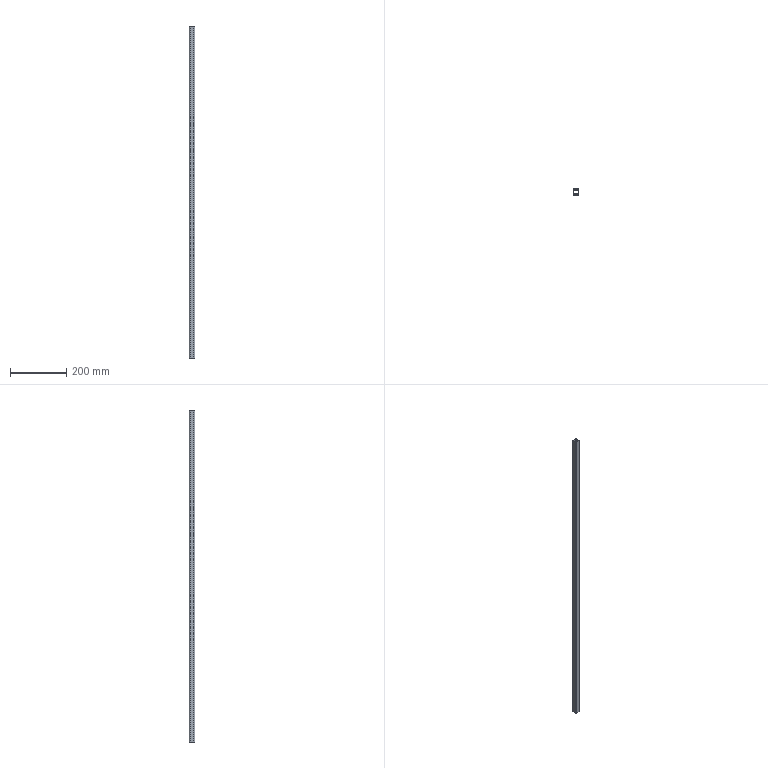Part | STEP file | DIN EN 10210-2 - 20 x 20 x 2 - 500 | 1 solid | 18 faces | box 20 x 20 x 1180 mm | volume 164855 mm3 | plane 10 | cylinder 8 | commonest cylinder face diameters 4 x4 6 x4
STEP:
#1=CARTESIAN_POINT('',(0.,0.,0.));
#2=DIRECTION('',(0.,0.,1.));
#3=DIRECTION('',(1.,0.,0.));
#4=AXIS2_PLACEMENT_3D('',#1,#2,#3);
#5=CARTESIAN_POINT('',(8.,6.,0.));
#6=VERTEX_POINT('',#5);
#7=CARTESIAN_POINT('',(8.,6.,1180.));
#8=VERTEX_POINT('',#7);
#9=CARTESIAN_POINT('',(8.,6.,0.));
#10=DIRECTION('',(0.,0.,1.));
#11=VECTOR('',#10,1.);
#12=LINE('',#9,#11);
#13=CARTESIAN_POINT('',(6.,6.,0.));
#14=DIRECTION('',(0.,0.,1.));
#15=DIRECTION('',(1.,0.,0.));
#16=AXIS2_PLACEMENT_3D('',#13,#14,#15);
#17=CYLINDRICAL_SURFACE('',#16,2.);
#18=CARTESIAN_POINT('',(0.,0.));
#19=DIRECTION('',(0.,1.));
#20=VECTOR('',#19,1.);
#21=LINE('',#18,#20);
#22=(GEOMETRIC_REPRESENTATION_CONTEXT(2)PARAMETRIC_REPRESENTATION_CONTEXT()REPRESENTATION_CONTEXT('',''));
#23=DEFINITIONAL_REPRESENTATION('',(#21),#22);
#24=PCURVE('',#17,#23);
#25=CARTESIAN_POINT('',(8.,6.,0.));
#26=DIRECTION('',(1.,0.,0.));
#27=DIRECTION('',(0.,0.,-1.));
#28=AXIS2_PLACEMENT_3D('',#25,#26,#27);
#29=PLANE('',#28);
#30=CARTESIAN_POINT('',(0.,0.));
#31=DIRECTION('',(-1.,0.));
#32=VECTOR('',#31,1.);
#33=LINE('',#30,#32);
#34=(GEOMETRIC_REPRESENTATION_CONTEXT(2)PARAMETRIC_REPRESENTATION_CONTEXT()REPRESENTATION_CONTEXT('',''));
#35=DEFINITIONAL_REPRESENTATION('',(#33),#34);
#36=PCURVE('',#29,#35);
#37=SURFACE_CURVE('',#12,(#24,#36),.PCURVE_S1.);
#38=EDGE_CURVE('',#6,#8,#37,.T.);
#39=ORIENTED_EDGE('',*,*,#38,.F.);
#40=CARTESIAN_POINT('',(6.,8.,0.));
#41=VERTEX_POINT('',#40);
#42=CARTESIAN_POINT('',(6.,6.,0.));
#43=DIRECTION('',(0.,0.,1.));
#44=DIRECTION('',(1.,0.,0.));
#45=AXIS2_PLACEMENT_3D('',#42,#43,#44);
#46=CIRCLE('',#45,2.);
#47=CARTESIAN_POINT('',(0.,0.));
#48=DIRECTION('',(1.,0.));
#49=VECTOR('',#48,1.);
#50=LINE('',#47,#49);
#51=(GEOMETRIC_REPRESENTATION_CONTEXT(2)PARAMETRIC_REPRESENTATION_CONTEXT()REPRESENTATION_CONTEXT('',''));
#52=DEFINITIONAL_REPRESENTATION('',(#50),#51);
#53=PCURVE('',#17,#52);
#54=CARTESIAN_POINT('',(0.,0.,0.));
#55=DIRECTION('',(0.,0.,1.));
#56=DIRECTION('',(1.,0.,0.));
#57=AXIS2_PLACEMENT_3D('',#54,#55,#56);
#58=PLANE('',#57);
#59=CARTESIAN_POINT('',(6.,6.));
#60=DIRECTION('',(1.,0.));
#61=AXIS2_PLACEMENT_2D('',#59,#60);
#62=CIRCLE('',#61,2.);
#63=(GEOMETRIC_REPRESENTATION_CONTEXT(2)PARAMETRIC_REPRESENTATION_CONTEXT()REPRESENTATION_CONTEXT('',''));
#64=DEFINITIONAL_REPRESENTATION('',(#62),#63);
#65=PCURVE('',#58,#64);
#66=SURFACE_CURVE('',#46,(#53,#65),.PCURVE_S1.);
#67=EDGE_CURVE('',#6,#41,#66,.T.);
#68=ORIENTED_EDGE('',*,*,#67,.T.);
#69=CARTESIAN_POINT('',(6.,8.,1180.));
#70=VERTEX_POINT('',#69);
#71=CARTESIAN_POINT('',(6.,8.,0.));
#72=DIRECTION('',(0.,0.,1.));
#73=VECTOR('',#72,1.);
#74=LINE('',#71,#73);
#75=CARTESIAN_POINT('',(1.571,0.));
#76=DIRECTION('',(0.,1.));
#77=VECTOR('',#76,1.);
#78=LINE('',#75,#77);
#79=(GEOMETRIC_REPRESENTATION_CONTEXT(2)PARAMETRIC_REPRESENTATION_CONTEXT()REPRESENTATION_CONTEXT('',''));
#80=DEFINITIONAL_REPRESENTATION('',(#78),#79);
#81=PCURVE('',#17,#80);
#82=CARTESIAN_POINT('',(-6.,8.,0.));
#83=DIRECTION('',(0.,1.,0.));
#84=DIRECTION('',(0.,0.,1.));
#85=AXIS2_PLACEMENT_3D('',#82,#83,#84);
#86=PLANE('',#85);
#87=CARTESIAN_POINT('',(0.,12.));
#88=DIRECTION('',(1.,0.));
#89=VECTOR('',#88,1.);
#90=LINE('',#87,#89);
#91=(GEOMETRIC_REPRESENTATION_CONTEXT(2)PARAMETRIC_REPRESENTATION_CONTEXT()REPRESENTATION_CONTEXT('',''));
#92=DEFINITIONAL_REPRESENTATION('',(#90),#91);
#93=PCURVE('',#86,#92);
#94=SURFACE_CURVE('',#74,(#81,#93),.PCURVE_S1.);
#95=EDGE_CURVE('',#41,#70,#94,.T.);
#96=ORIENTED_EDGE('',*,*,#95,.T.);
#97=CARTESIAN_POINT('',(6.,6.,1180.));
#98=DIRECTION('',(0.,0.,1.));
#99=DIRECTION('',(1.,0.,0.));
#100=AXIS2_PLACEMENT_3D('',#97,#98,#99);
#101=CIRCLE('',#100,2.);
#102=CARTESIAN_POINT('',(0.,1180.));
#103=DIRECTION('',(1.,0.));
#104=VECTOR('',#103,1.);
#105=LINE('',#102,#104);
#106=(GEOMETRIC_REPRESENTATION_CONTEXT(2)PARAMETRIC_REPRESENTATION_CONTEXT()REPRESENTATION_CONTEXT('',''));
#107=DEFINITIONAL_REPRESENTATION('',(#105),#106);
#108=PCURVE('',#17,#107);
#109=CARTESIAN_POINT('',(0.,0.,1180.));
#110=DIRECTION('',(0.,0.,1.));
#111=DIRECTION('',(1.,0.,0.));
#112=AXIS2_PLACEMENT_3D('',#109,#110,#111);
#113=PLANE('',#112);
#114=CARTESIAN_POINT('',(6.,6.));
#115=DIRECTION('',(1.,0.));
#116=AXIS2_PLACEMENT_2D('',#114,#115);
#117=CIRCLE('',#116,2.);
#118=(GEOMETRIC_REPRESENTATION_CONTEXT(2)PARAMETRIC_REPRESENTATION_CONTEXT()REPRESENTATION_CONTEXT('',''));
#119=DEFINITIONAL_REPRESENTATION('',(#117),#118);
#120=PCURVE('',#113,#119);
#121=SURFACE_CURVE('',#101,(#108,#120),.PCURVE_S1.);
#122=EDGE_CURVE('',#8,#70,#121,.T.);
#123=ORIENTED_EDGE('',*,*,#122,.F.);
#124=EDGE_LOOP('',(#39,#68,#96,#123));
#125=FACE_BOUND('',#124,.F.);
#126=ADVANCED_FACE('',(#125),#17,.F.);
#127=CARTESIAN_POINT('',(-6.,8.,1180.));
#128=VERTEX_POINT('',#127);
#129=CARTESIAN_POINT('',(-3.,8.,1180.));
#130=DIRECTION('',(-1.,0.,0.));
#131=VECTOR('',#130,1.);
#132=LINE('',#129,#131);
#133=CARTESIAN_POINT('',(1180.,3.));
#134=DIRECTION('',(0.,-1.));
#135=VECTOR('',#134,1.);
#136=LINE('',#133,#135);
#137=(GEOMETRIC_REPRESENTATION_CONTEXT(2)PARAMETRIC_REPRESENTATION_CONTEXT()REPRESENTATION_CONTEXT('',''));
#138=DEFINITIONAL_REPRESENTATION('',(#136),#137);
#139=PCURVE('',#86,#138);
#140=CARTESIAN_POINT('',(-3.,8.));
#141=DIRECTION('',(-1.,0.));
#142=VECTOR('',#141,1.);
#143=LINE('',#140,#142);
#144=(GEOMETRIC_REPRESENTATION_CONTEXT(2)PARAMETRIC_REPRESENTATION_CONTEXT()REPRESENTATION_CONTEXT('',''));
#145=DEFINITIONAL_REPRESENTATION('',(#143),#144);
#146=PCURVE('',#113,#145);
#147=SURFACE_CURVE('',#132,(#139,#146),.PCURVE_S1.);
#148=EDGE_CURVE('',#70,#128,#147,.T.);
#149=ORIENTED_EDGE('',*,*,#148,.T.);
#150=CARTESIAN_POINT('',(-6.,8.,0.));
#151=VERTEX_POINT('',#150);
#152=CARTESIAN_POINT('',(-6.,8.,0.));
#153=DIRECTION('',(0.,0.,1.));
#154=VECTOR('',#153,1.);
#155=LINE('',#152,#154);
#156=CARTESIAN_POINT('',(0.,0.));
#157=DIRECTION('',(1.,0.));
#158=VECTOR('',#157,1.);
#159=LINE('',#156,#158);
#160=(GEOMETRIC_REPRESENTATION_CONTEXT(2)PARAMETRIC_REPRESENTATION_CONTEXT()REPRESENTATION_CONTEXT('',''));
#161=DEFINITIONAL_REPRESENTATION('',(#159),#160);
#162=PCURVE('',#86,#161);
#163=CARTESIAN_POINT('',(-6.,6.,0.));
#164=DIRECTION('',(0.,0.,1.));
#165=DIRECTION('',(0.,1.,0.));
#166=AXIS2_PLACEMENT_3D('',#163,#164,#165);
#167=CYLINDRICAL_SURFACE('',#166,2.);
#168=CARTESIAN_POINT('',(0.,0.));
#169=DIRECTION('',(0.,1.));
#170=VECTOR('',#169,1.);
#171=LINE('',#168,#170);
#172=(GEOMETRIC_REPRESENTATION_CONTEXT(2)PARAMETRIC_REPRESENTATION_CONTEXT()REPRESENTATION_CONTEXT('',''));
#173=DEFINITIONAL_REPRESENTATION('',(#171),#172);
#174=PCURVE('',#167,#173);
#175=SURFACE_CURVE('',#155,(#162,#174),.PCURVE_S1.);
#176=EDGE_CURVE('',#151,#128,#175,.T.);
#177=ORIENTED_EDGE('',*,*,#176,.F.);
#178=CARTESIAN_POINT('',(-3.,8.,0.));
#179=DIRECTION('',(-1.,0.,0.));
#180=VECTOR('',#179,1.);
#181=LINE('',#178,#180);
#182=CARTESIAN_POINT('',(0.,3.));
#183=DIRECTION('',(0.,-1.));
#184=VECTOR('',#183,1.);
#185=LINE('',#182,#184);
#186=(GEOMETRIC_REPRESENTATION_CONTEXT(2)PARAMETRIC_REPRESENTATION_CONTEXT()REPRESENTATION_CONTEXT('',''));
#187=DEFINITIONAL_REPRESENTATION('',(#185),#186);
#188=PCURVE('',#86,#187);
#189=CARTESIAN_POINT('',(-3.,8.));
#190=DIRECTION('',(-1.,0.));
#191=VECTOR('',#190,1.);
#192=LINE('',#189,#191);
#193=(GEOMETRIC_REPRESENTATION_CONTEXT(2)PARAMETRIC_REPRESENTATION_CONTEXT()REPRESENTATION_CONTEXT('',''));
#194=DEFINITIONAL_REPRESENTATION('',(#192),#193);
#195=PCURVE('',#58,#194);
#196=SURFACE_CURVE('',#181,(#188,#195),.PCURVE_S1.);
#197=EDGE_CURVE('',#41,#151,#196,.T.);
#198=ORIENTED_EDGE('',*,*,#197,.F.);
#199=ORIENTED_EDGE('',*,*,#95,.T.);
#200=EDGE_LOOP('',(#149,#177,#198,#199));
#201=FACE_BOUND('',#200,.T.);
#202=ADVANCED_FACE('',(#201),#86,.F.);
#203=ORIENTED_EDGE('',*,*,#176,.F.);
#204=CARTESIAN_POINT('',(-8.,6.,0.));
#205=VERTEX_POINT('',#204);
#206=CARTESIAN_POINT('',(-6.,6.,0.));
#207=DIRECTION('',(0.,0.,1.));
#208=DIRECTION('',(0.,1.,0.));
#209=AXIS2_PLACEMENT_3D('',#206,#207,#208);
#210=CIRCLE('',#209,2.);
#211=CARTESIAN_POINT('',(0.,0.));
#212=DIRECTION('',(1.,0.));
#213=VECTOR('',#212,1.);
#214=LINE('',#211,#213);
#215=(GEOMETRIC_REPRESENTATION_CONTEXT(2)PARAMETRIC_REPRESENTATION_CONTEXT()REPRESENTATION_CONTEXT('',''));
#216=DEFINITIONAL_REPRESENTATION('',(#214),#215);
#217=PCURVE('',#167,#216);
#218=CARTESIAN_POINT('',(-6.,6.));
#219=DIRECTION('',(0.,1.));
#220=AXIS2_PLACEMENT_2D('',#218,#219);
#221=CIRCLE('',#220,2.);
#222=(GEOMETRIC_REPRESENTATION_CONTEXT(2)PARAMETRIC_REPRESENTATION_CONTEXT()REPRESENTATION_CONTEXT('',''));
#223=DEFINITIONAL_REPRESENTATION('',(#221),#222);
#224=PCURVE('',#58,#223);
#225=SURFACE_CURVE('',#210,(#217,#224),.PCURVE_S1.);
#226=EDGE_CURVE('',#151,#205,#225,.T.);
#227=ORIENTED_EDGE('',*,*,#226,.T.);
#228=CARTESIAN_POINT('',(-8.,6.,1180.));
#229=VERTEX_POINT('',#228);
#230=CARTESIAN_POINT('',(-8.,6.,0.));
#231=DIRECTION('',(0.,0.,1.));
#232=VECTOR('',#231,1.);
#233=LINE('',#230,#232);
#234=CARTESIAN_POINT('',(1.571,0.));
#235=DIRECTION('',(0.,1.));
#236=VECTOR('',#235,1.);
#237=LINE('',#234,#236);
#238=(GEOMETRIC_REPRESENTATION_CONTEXT(2)PARAMETRIC_REPRESENTATION_CONTEXT()REPRESENTATION_CONTEXT('',''));
#239=DEFINITIONAL_REPRESENTATION('',(#237),#238);
#240=PCURVE('',#167,#239);
#241=CARTESIAN_POINT('',(-8.,-6.,0.));
#242=DIRECTION('',(-1.,0.,0.));
#243=DIRECTION('',(0.,0.,1.));
#244=AXIS2_PLACEMENT_3D('',#241,#242,#243);
#245=PLANE('',#244);
#246=CARTESIAN_POINT('',(0.,12.));
#247=DIRECTION('',(1.,0.));
#248=VECTOR('',#247,1.);
#249=LINE('',#246,#248);
#250=(GEOMETRIC_REPRESENTATION_CONTEXT(2)PARAMETRIC_REPRESENTATION_CONTEXT()REPRESENTATION_CONTEXT('',''));
#251=DEFINITIONAL_REPRESENTATION('',(#249),#250);
#252=PCURVE('',#245,#251);
#253=SURFACE_CURVE('',#233,(#240,#252),.PCURVE_S1.);
#254=EDGE_CURVE('',#205,#229,#253,.T.);
#255=ORIENTED_EDGE('',*,*,#254,.T.);
#256=CARTESIAN_POINT('',(-6.,6.,1180.));
#257=DIRECTION('',(0.,0.,1.));
#258=DIRECTION('',(0.,1.,0.));
#259=AXIS2_PLACEMENT_3D('',#256,#257,#258);
#260=CIRCLE('',#259,2.);
#261=CARTESIAN_POINT('',(0.,1180.));
#262=DIRECTION('',(1.,0.));
#263=VECTOR('',#262,1.);
#264=LINE('',#261,#263);
#265=(GEOMETRIC_REPRESENTATION_CONTEXT(2)PARAMETRIC_REPRESENTATION_CONTEXT()REPRESENTATION_CONTEXT('',''));
#266=DEFINITIONAL_REPRESENTATION('',(#264),#265);
#267=PCURVE('',#167,#266);
#268=CARTESIAN_POINT('',(-6.,6.));
#269=DIRECTION('',(0.,1.));
#270=AXIS2_PLACEMENT_2D('',#268,#269);
#271=CIRCLE('',#270,2.);
#272=(GEOMETRIC_REPRESENTATION_CONTEXT(2)PARAMETRIC_REPRESENTATION_CONTEXT()REPRESENTATION_CONTEXT('',''));
#273=DEFINITIONAL_REPRESENTATION('',(#271),#272);
#274=PCURVE('',#113,#273);
#275=SURFACE_CURVE('',#260,(#267,#274),.PCURVE_S1.);
#276=EDGE_CURVE('',#128,#229,#275,.T.);
#277=ORIENTED_EDGE('',*,*,#276,.F.);
#278=EDGE_LOOP('',(#203,#227,#255,#277));
#279=FACE_BOUND('',#278,.F.);
#280=ADVANCED_FACE('',(#279),#167,.F.);
#281=CARTESIAN_POINT('',(-8.,-6.,1180.));
#282=VERTEX_POINT('',#281);
#283=CARTESIAN_POINT('',(-8.,-3.,1180.));
#284=DIRECTION('',(0.,-1.,0.));
#285=VECTOR('',#284,1.);
#286=LINE('',#283,#285);
#287=CARTESIAN_POINT('',(1180.,3.));
#288=DIRECTION('',(0.,-1.));
#289=VECTOR('',#288,1.);
#290=LINE('',#287,#289);
#291=(GEOMETRIC_REPRESENTATION_CONTEXT(2)PARAMETRIC_REPRESENTATION_CONTEXT()REPRESENTATION_CONTEXT('',''));
#292=DEFINITIONAL_REPRESENTATION('',(#290),#291);
#293=PCURVE('',#245,#292);
#294=CARTESIAN_POINT('',(-8.,-3.));
#295=DIRECTION('',(0.,-1.));
#296=VECTOR('',#295,1.);
#297=LINE('',#294,#296);
#298=(GEOMETRIC_REPRESENTATION_CONTEXT(2)PARAMETRIC_REPRESENTATION_CONTEXT()REPRESENTATION_CONTEXT('',''));
#299=DEFINITIONAL_REPRESENTATION('',(#297),#298);
#300=PCURVE('',#113,#299);
#301=SURFACE_CURVE('',#286,(#293,#300),.PCURVE_S1.);
#302=EDGE_CURVE('',#229,#282,#301,.T.);
#303=ORIENTED_EDGE('',*,*,#302,.T.);
#304=CARTESIAN_POINT('',(-8.,-6.,0.));
#305=VERTEX_POINT('',#304);
#306=CARTESIAN_POINT('',(-8.,-6.,0.));
#307=DIRECTION('',(0.,0.,1.));
#308=VECTOR('',#307,1.);
#309=LINE('',#306,#308);
#310=CARTESIAN_POINT('',(0.,0.));
#311=DIRECTION('',(1.,0.));
#312=VECTOR('',#311,1.);
#313=LINE('',#310,#312);
#314=(GEOMETRIC_REPRESENTATION_CONTEXT(2)PARAMETRIC_REPRESENTATION_CONTEXT()REPRESENTATION_CONTEXT('',''));
#315=DEFINITIONAL_REPRESENTATION('',(#313),#314);
#316=PCURVE('',#245,#315);
#317=CARTESIAN_POINT('',(-6.,-6.,0.));
#318=DIRECTION('',(0.,0.,1.));
#319=DIRECTION('',(-1.,0.,0.));
#320=AXIS2_PLACEMENT_3D('',#317,#318,#319);
#321=CYLINDRICAL_SURFACE('',#320,2.);
#322=CARTESIAN_POINT('',(0.,0.));
#323=DIRECTION('',(0.,1.));
#324=VECTOR('',#323,1.);
#325=LINE('',#322,#324);
#326=(GEOMETRIC_REPRESENTATION_CONTEXT(2)PARAMETRIC_REPRESENTATION_CONTEXT()REPRESENTATION_CONTEXT('',''));
#327=DEFINITIONAL_REPRESENTATION('',(#325),#326);
#328=PCURVE('',#321,#327);
#329=SURFACE_CURVE('',#309,(#316,#328),.PCURVE_S1.);
#330=EDGE_CURVE('',#305,#282,#329,.T.);
#331=ORIENTED_EDGE('',*,*,#330,.F.);
#332=CARTESIAN_POINT('',(-8.,-3.,0.));
#333=DIRECTION('',(0.,-1.,0.));
#334=VECTOR('',#333,1.);
#335=LINE('',#332,#334);
#336=CARTESIAN_POINT('',(0.,3.));
#337=DIRECTION('',(0.,-1.));
#338=VECTOR('',#337,1.);
#339=LINE('',#336,#338);
#340=(GEOMETRIC_REPRESENTATION_CONTEXT(2)PARAMETRIC_REPRESENTATION_CONTEXT()REPRESENTATION_CONTEXT('',''));
#341=DEFINITIONAL_REPRESENTATION('',(#339),#340);
#342=PCURVE('',#245,#341);
#343=CARTESIAN_POINT('',(-8.,-3.));
#344=DIRECTION('',(0.,-1.));
#345=VECTOR('',#344,1.);
#346=LINE('',#343,#345);
#347=(GEOMETRIC_REPRESENTATION_CONTEXT(2)PARAMETRIC_REPRESENTATION_CONTEXT()REPRESENTATION_CONTEXT('',''));
#348=DEFINITIONAL_REPRESENTATION('',(#346),#347);
#349=PCURVE('',#58,#348);
#350=SURFACE_CURVE('',#335,(#342,#349),.PCURVE_S1.);
#351=EDGE_CURVE('',#205,#305,#350,.T.);
#352=ORIENTED_EDGE('',*,*,#351,.F.);
#353=ORIENTED_EDGE('',*,*,#254,.T.);
#354=EDGE_LOOP('',(#303,#331,#352,#353));
#355=FACE_BOUND('',#354,.T.);
#356=ADVANCED_FACE('',(#355),#245,.F.);
#357=CARTESIAN_POINT('',(10.,7.,1180.));
#358=VERTEX_POINT('',#357);
#359=CARTESIAN_POINT('',(10.,-7.,1180.));
#360=VERTEX_POINT('',#359);
#361=CARTESIAN_POINT('',(10.,3.5,1180.));
#362=DIRECTION('',(0.,-1.,0.));
#363=VECTOR('',#362,1.);
#364=LINE('',#361,#363);
#365=CARTESIAN_POINT('',(10.,7.,0.));
#366=DIRECTION('',(1.,0.,0.));
#367=DIRECTION('',(0.,0.,-1.));
#368=AXIS2_PLACEMENT_3D('',#365,#366,#367);
#369=PLANE('',#368);
#370=CARTESIAN_POINT('',(-1180.,-3.5));
#371=DIRECTION('',(0.,-1.));
#372=VECTOR('',#371,1.);
#373=LINE('',#370,#372);
#374=(GEOMETRIC_REPRESENTATION_CONTEXT(2)PARAMETRIC_REPRESENTATION_CONTEXT()REPRESENTATION_CONTEXT('',''));
#375=DEFINITIONAL_REPRESENTATION('',(#373),#374);
#376=PCURVE('',#369,#375);
#377=CARTESIAN_POINT('',(10.,3.5));
#378=DIRECTION('',(0.,-1.));
#379=VECTOR('',#378,1.);
#380=LINE('',#377,#379);
#381=(GEOMETRIC_REPRESENTATION_CONTEXT(2)PARAMETRIC_REPRESENTATION_CONTEXT()REPRESENTATION_CONTEXT('',''));
#382=DEFINITIONAL_REPRESENTATION('',(#380),#381);
#383=PCURVE('',#113,#382);
#384=SURFACE_CURVE('',#364,(#376,#383),.PCURVE_S1.);
#385=EDGE_CURVE('',#358,#360,#384,.T.);
#386=ORIENTED_EDGE('',*,*,#385,.T.);
#387=CARTESIAN_POINT('',(10.,-7.,0.));
#388=VERTEX_POINT('',#387);
#389=CARTESIAN_POINT('',(10.,-7.,0.));
#390=DIRECTION('',(0.,0.,1.));
#391=VECTOR('',#390,1.);
#392=LINE('',#389,#391);
#393=CARTESIAN_POINT('',(0.,-14.));
#394=DIRECTION('',(-1.,0.));
#395=VECTOR('',#394,1.);
#396=LINE('',#393,#395);
#397=(GEOMETRIC_REPRESENTATION_CONTEXT(2)PARAMETRIC_REPRESENTATION_CONTEXT()REPRESENTATION_CONTEXT('',''));
#398=DEFINITIONAL_REPRESENTATION('',(#396),#397);
#399=PCURVE('',#369,#398);
#400=CARTESIAN_POINT('',(7.,-7.,0.));
#401=DIRECTION('',(0.,0.,1.));
#402=DIRECTION('',(0.,1.,0.));
#403=AXIS2_PLACEMENT_3D('',#400,#401,#402);
#404=CYLINDRICAL_SURFACE('',#403,3.);
#405=CARTESIAN_POINT('',(4.712,0.));
#406=DIRECTION('',(0.,1.));
#407=VECTOR('',#406,1.);
#408=LINE('',#405,#407);
#409=(GEOMETRIC_REPRESENTATION_CONTEXT(2)PARAMETRIC_REPRESENTATION_CONTEXT()REPRESENTATION_CONTEXT('',''));
#410=DEFINITIONAL_REPRESENTATION('',(#408),#409);
#411=PCURVE('',#404,#410);
#412=SURFACE_CURVE('',#392,(#399,#411),.PCURVE_S1.);
#413=EDGE_CURVE('',#388,#360,#412,.T.);
#414=ORIENTED_EDGE('',*,*,#413,.F.);
#415=CARTESIAN_POINT('',(10.,7.,0.));
#416=VERTEX_POINT('',#415);
#417=CARTESIAN_POINT('',(10.,3.5,0.));
#418=DIRECTION('',(0.,-1.,0.));
#419=VECTOR('',#418,1.);
#420=LINE('',#417,#419);
#421=CARTESIAN_POINT('',(0.,-3.5));
#422=DIRECTION('',(0.,-1.));
#423=VECTOR('',#422,1.);
#424=LINE('',#421,#423);
#425=(GEOMETRIC_REPRESENTATION_CONTEXT(2)PARAMETRIC_REPRESENTATION_CONTEXT()REPRESENTATION_CONTEXT('',''));
#426=DEFINITIONAL_REPRESENTATION('',(#424),#425);
#427=PCURVE('',#369,#426);
#428=CARTESIAN_POINT('',(10.,3.5));
#429=DIRECTION('',(0.,-1.));
#430=VECTOR('',#429,1.);
#431=LINE('',#428,#430);
#432=(GEOMETRIC_REPRESENTATION_CONTEXT(2)PARAMETRIC_REPRESENTATION_CONTEXT()REPRESENTATION_CONTEXT('',''));
#433=DEFINITIONAL_REPRESENTATION('',(#431),#432);
#434=PCURVE('',#58,#433);
#435=SURFACE_CURVE('',#420,(#427,#434),.PCURVE_S1.);
#436=EDGE_CURVE('',#416,#388,#435,.T.);
#437=ORIENTED_EDGE('',*,*,#436,.F.);
#438=CARTESIAN_POINT('',(10.,7.,0.));
#439=DIRECTION('',(0.,0.,1.));
#440=VECTOR('',#439,1.);
#441=LINE('',#438,#440);
#442=CARTESIAN_POINT('',(0.,0.));
#443=DIRECTION('',(-1.,0.));
#444=VECTOR('',#443,1.);
#445=LINE('',#442,#444);
#446=(GEOMETRIC_REPRESENTATION_CONTEXT(2)PARAMETRIC_REPRESENTATION_CONTEXT()REPRESENTATION_CONTEXT('',''));
#447=DEFINITIONAL_REPRESENTATION('',(#445),#446);
#448=PCURVE('',#369,#447);
#449=CARTESIAN_POINT('',(7.,7.,0.));
#450=DIRECTION('',(0.,0.,1.));
#451=DIRECTION('',(-1.,0.,0.));
#452=AXIS2_PLACEMENT_3D('',#449,#450,#451);
#453=CYLINDRICAL_SURFACE('',#452,3.);
#454=CARTESIAN_POINT('',(3.142,0.));
#455=DIRECTION('',(0.,1.));
#456=VECTOR('',#455,1.);
#457=LINE('',#454,#456);
#458=(GEOMETRIC_REPRESENTATION_CONTEXT(2)PARAMETRIC_REPRESENTATION_CONTEXT()REPRESENTATION_CONTEXT('',''));
#459=DEFINITIONAL_REPRESENTATION('',(#457),#458);
#460=PCURVE('',#453,#459);
#461=SURFACE_CURVE('',#441,(#448,#460),.PCURVE_S1.);
#462=EDGE_CURVE('',#416,#358,#461,.T.);
#463=ORIENTED_EDGE('',*,*,#462,.T.);
#464=EDGE_LOOP('',(#386,#414,#437,#463));
#465=FACE_BOUND('',#464,.T.);
#466=ADVANCED_FACE('',(#465),#369,.T.);
#467=CARTESIAN_POINT('',(7.,-10.,1180.));
#468=VERTEX_POINT('',#467);
#469=CARTESIAN_POINT('',(7.,-7.,1180.));
#470=DIRECTION('',(0.,0.,-1.));
#471=DIRECTION('',(0.,1.,0.));
#472=AXIS2_PLACEMENT_3D('',#469,#470,#471);
#473=CIRCLE('',#472,3.);
#474=CARTESIAN_POINT('',(6.283,1180.));
#475=DIRECTION('',(-1.,0.));
#476=VECTOR('',#475,1.);
#477=LINE('',#474,#476);
#478=(GEOMETRIC_REPRESENTATION_CONTEXT(2)PARAMETRIC_REPRESENTATION_CONTEXT()REPRESENTATION_CONTEXT('',''));
#479=DEFINITIONAL_REPRESENTATION('',(#477),#478);
#480=PCURVE('',#404,#479);
#481=CARTESIAN_POINT('',(7.,-4.));
#482=CARTESIAN_POINT('',(12.196,-4.));
#483=CARTESIAN_POINT('',(9.598,-8.5));
#484=CARTESIAN_POINT('',(7.,-13.));
#485=CARTESIAN_POINT('',(4.402,-8.5));
#486=CARTESIAN_POINT('',(1.804,-4.));
#487=CARTESIAN_POINT('',(7.,-4.));
#488=(BOUNDED_CURVE()B_SPLINE_CURVE(2,(#481,#482,#483,#484,#485,#486,#487),.UNSPECIFIED.,.T.,.F.)B_SPLINE_CURVE_WITH_KNOTS((1,2,2,2,2,1),(-2.094,0.,2.094,4.189,6.283,8.378),.UNSPECIFIED.)CURVE()GEOMETRIC_REPRESENTATION_ITEM()RATIONAL_B_SPLINE_CURVE((1.,0.5,1.,0.5,1.,0.5,1.))REPRESENTATION_ITEM(''));
#489=(GEOMETRIC_REPRESENTATION_CONTEXT(2)PARAMETRIC_REPRESENTATION_CONTEXT()REPRESENTATION_CONTEXT('',''));
#490=DEFINITIONAL_REPRESENTATION('',(#488),#489);
#491=PCURVE('',#113,#490);
#492=SURFACE_CURVE('',#473,(#480,#491),.PCURVE_S1.);
#493=EDGE_CURVE('',#360,#468,#492,.T.);
#494=ORIENTED_EDGE('',*,*,#493,.T.);
#495=CARTESIAN_POINT('',(7.,-10.,0.));
#496=VERTEX_POINT('',#495);
#497=CARTESIAN_POINT('',(7.,-10.,0.));
#498=DIRECTION('',(0.,0.,1.));
#499=VECTOR('',#498,1.);
#500=LINE('',#497,#499);
#501=CARTESIAN_POINT('',(3.142,0.));
#502=DIRECTION('',(0.,1.));
#503=VECTOR('',#502,1.);
#504=LINE('',#501,#503);
#505=(GEOMETRIC_REPRESENTATION_CONTEXT(2)PARAMETRIC_REPRESENTATION_CONTEXT()REPRESENTATION_CONTEXT('',''));
#506=DEFINITIONAL_REPRESENTATION('',(#504),#505);
#507=PCURVE('',#404,#506);
#508=CARTESIAN_POINT('',(7.,-10.,0.));
#509=DIRECTION('',(0.,-1.,0.));
#510=DIRECTION('',(0.,0.,-1.));
#511=AXIS2_PLACEMENT_3D('',#508,#509,#510);
#512=PLANE('',#511);
#513=CARTESIAN_POINT('',(0.,0.));
#514=DIRECTION('',(-1.,0.));
#515=VECTOR('',#514,1.);
#516=LINE('',#513,#515);
#517=(GEOMETRIC_REPRESENTATION_CONTEXT(2)PARAMETRIC_REPRESENTATION_CONTEXT()REPRESENTATION_CONTEXT('',''));
#518=DEFINITIONAL_REPRESENTATION('',(#516),#517);
#519=PCURVE('',#512,#518);
#520=SURFACE_CURVE('',#500,(#507,#519),.PCURVE_S1.);
#521=EDGE_CURVE('',#496,#468,#520,.T.);
#522=ORIENTED_EDGE('',*,*,#521,.F.);
#523=CARTESIAN_POINT('',(7.,-7.,0.));
#524=DIRECTION('',(0.,0.,-1.));
#525=DIRECTION('',(0.,1.,0.));
#526=AXIS2_PLACEMENT_3D('',#523,#524,#525);
#527=CIRCLE('',#526,3.);
#528=CARTESIAN_POINT('',(6.283,0.));
#529=DIRECTION('',(-1.,0.));
#530=VECTOR('',#529,1.);
#531=LINE('',#528,#530);
#532=(GEOMETRIC_REPRESENTATION_CONTEXT(2)PARAMETRIC_REPRESENTATION_CONTEXT()REPRESENTATION_CONTEXT('',''));
#533=DEFINITIONAL_REPRESENTATION('',(#531),#532);
#534=PCURVE('',#404,#533);
#535=CARTESIAN_POINT('',(7.,-4.));
#536=CARTESIAN_POINT('',(12.196,-4.));
#537=CARTESIAN_POINT('',(9.598,-8.5));
#538=CARTESIAN_POINT('',(7.,-13.));
#539=CARTESIAN_POINT('',(4.402,-8.5));
#540=CARTESIAN_POINT('',(1.804,-4.));
#541=CARTESIAN_POINT('',(7.,-4.));
#542=(BOUNDED_CURVE()B_SPLINE_CURVE(2,(#535,#536,#537,#538,#539,#540,#541),.UNSPECIFIED.,.T.,.F.)B_SPLINE_CURVE_WITH_KNOTS((1,2,2,2,2,1),(-2.094,0.,2.094,4.189,6.283,8.378),.UNSPECIFIED.)CURVE()GEOMETRIC_REPRESENTATION_ITEM()RATIONAL_B_SPLINE_CURVE((1.,0.5,1.,0.5,1.,0.5,1.))REPRESENTATION_ITEM(''));
#543=(GEOMETRIC_REPRESENTATION_CONTEXT(2)PARAMETRIC_REPRESENTATION_CONTEXT()REPRESENTATION_CONTEXT('',''));
#544=DEFINITIONAL_REPRESENTATION('',(#542),#543);
#545=PCURVE('',#58,#544);
#546=SURFACE_CURVE('',#527,(#534,#545),.PCURVE_S1.);
#547=EDGE_CURVE('',#388,#496,#546,.T.);
#548=ORIENTED_EDGE('',*,*,#547,.F.);
#549=ORIENTED_EDGE('',*,*,#413,.T.);
#550=EDGE_LOOP('',(#494,#522,#548,#549));
#551=FACE_BOUND('',#550,.T.);
#552=ADVANCED_FACE('',(#551),#404,.T.);
#553=CARTESIAN_POINT('',(-7.,-10.,1180.));
#554=VERTEX_POINT('',#553);
#555=CARTESIAN_POINT('',(3.5,-10.,1180.));
#556=DIRECTION('',(-1.,0.,0.));
#557=VECTOR('',#556,1.);
#558=LINE('',#555,#557);
#559=CARTESIAN_POINT('',(-1180.,-3.5));
#560=DIRECTION('',(0.,-1.));
#561=VECTOR('',#560,1.);
#562=LINE('',#559,#561);
#563=(GEOMETRIC_REPRESENTATION_CONTEXT(2)PARAMETRIC_REPRESENTATION_CONTEXT()REPRESENTATION_CONTEXT('',''));
#564=DEFINITIONAL_REPRESENTATION('',(#562),#563);
#565=PCURVE('',#512,#564);
#566=CARTESIAN_POINT('',(3.5,-10.));
#567=DIRECTION('',(-1.,0.));
#568=VECTOR('',#567,1.);
#569=LINE('',#566,#568);
#570=(GEOMETRIC_REPRESENTATION_CONTEXT(2)PARAMETRIC_REPRESENTATION_CONTEXT()REPRESENTATION_CONTEXT('',''));
#571=DEFINITIONAL_REPRESENTATION('',(#569),#570);
#572=PCURVE('',#113,#571);
#573=SURFACE_CURVE('',#558,(#565,#572),.PCURVE_S1.);
#574=EDGE_CURVE('',#468,#554,#573,.T.);
#575=ORIENTED_EDGE('',*,*,#574,.T.);
#576=CARTESIAN_POINT('',(-7.,-10.,0.));
#577=VERTEX_POINT('',#576);
#578=CARTESIAN_POINT('',(-7.,-10.,0.));
#579=DIRECTION('',(0.,0.,1.));
#580=VECTOR('',#579,1.);
#581=LINE('',#578,#580);
#582=CARTESIAN_POINT('',(0.,-14.));
#583=DIRECTION('',(-1.,0.));
#584=VECTOR('',#583,1.);
#585=LINE('',#582,#584);
#586=(GEOMETRIC_REPRESENTATION_CONTEXT(2)PARAMETRIC_REPRESENTATION_CONTEXT()REPRESENTATION_CONTEXT('',''));
#587=DEFINITIONAL_REPRESENTATION('',(#585),#586);
#588=PCURVE('',#512,#587);
#589=CARTESIAN_POINT('',(-7.,-7.,0.));
#590=DIRECTION('',(0.,0.,1.));
#591=DIRECTION('',(1.,0.,0.));
#592=AXIS2_PLACEMENT_3D('',#589,#590,#591);
#593=CYLINDRICAL_SURFACE('',#592,3.);
#594=CARTESIAN_POINT('',(4.712,0.));
#595=DIRECTION('',(0.,1.));
#596=VECTOR('',#595,1.);
#597=LINE('',#594,#596);
#598=(GEOMETRIC_REPRESENTATION_CONTEXT(2)PARAMETRIC_REPRESENTATION_CONTEXT()REPRESENTATION_CONTEXT('',''));
#599=DEFINITIONAL_REPRESENTATION('',(#597),#598);
#600=PCURVE('',#593,#599);
#601=SURFACE_CURVE('',#581,(#588,#600),.PCURVE_S1.);
#602=EDGE_CURVE('',#577,#554,#601,.T.);
#603=ORIENTED_EDGE('',*,*,#602,.F.);
#604=CARTESIAN_POINT('',(3.5,-10.,0.));
#605=DIRECTION('',(-1.,0.,0.));
#606=VECTOR('',#605,1.);
#607=LINE('',#604,#606);
#608=CARTESIAN_POINT('',(0.,-3.5));
#609=DIRECTION('',(0.,-1.));
#610=VECTOR('',#609,1.);
#611=LINE('',#608,#610);
#612=(GEOMETRIC_REPRESENTATION_CONTEXT(2)PARAMETRIC_REPRESENTATION_CONTEXT()REPRESENTATION_CONTEXT('',''));
#613=DEFINITIONAL_REPRESENTATION('',(#611),#612);
#614=PCURVE('',#512,#613);
#615=CARTESIAN_POINT('',(3.5,-10.));
#616=DIRECTION('',(-1.,0.));
#617=VECTOR('',#616,1.);
#618=LINE('',#615,#617);
#619=(GEOMETRIC_REPRESENTATION_CONTEXT(2)PARAMETRIC_REPRESENTATION_CONTEXT()REPRESENTATION_CONTEXT('',''));
#620=DEFINITIONAL_REPRESENTATION('',(#618),#619);
#621=PCURVE('',#58,#620);
#622=SURFACE_CURVE('',#607,(#614,#621),.PCURVE_S1.);
#623=EDGE_CURVE('',#496,#577,#622,.T.);
#624=ORIENTED_EDGE('',*,*,#623,.F.);
#625=ORIENTED_EDGE('',*,*,#521,.T.);
#626=EDGE_LOOP('',(#575,#603,#624,#625));
#627=FACE_BOUND('',#626,.T.);
#628=ADVANCED_FACE('',(#627),#512,.T.);
#629=CARTESIAN_POINT('',(-10.,-7.,1180.));
#630=VERTEX_POINT('',#629);
#631=CARTESIAN_POINT('',(-7.,-7.,1180.));
#632=DIRECTION('',(0.,0.,-1.));
#633=DIRECTION('',(1.,0.,0.));
#634=AXIS2_PLACEMENT_3D('',#631,#632,#633);
#635=CIRCLE('',#634,3.);
#636=CARTESIAN_POINT('',(6.283,1180.));
#637=DIRECTION('',(-1.,0.));
#638=VECTOR('',#637,1.);
#639=LINE('',#636,#638);
#640=(GEOMETRIC_REPRESENTATION_CONTEXT(2)PARAMETRIC_REPRESENTATION_CONTEXT()REPRESENTATION_CONTEXT('',''));
#641=DEFINITIONAL_REPRESENTATION('',(#639),#640);
#642=PCURVE('',#593,#641);
#643=CARTESIAN_POINT('',(-4.,-7.));
#644=CARTESIAN_POINT('',(-4.,-12.196));
#645=CARTESIAN_POINT('',(-8.5,-9.598));
#646=CARTESIAN_POINT('',(-13.,-7.));
#647=CARTESIAN_POINT('',(-8.5,-4.402));
#648=CARTESIAN_POINT('',(-4.,-1.804));
#649=CARTESIAN_POINT('',(-4.,-7.));
#650=(BOUNDED_CURVE()B_SPLINE_CURVE(2,(#643,#644,#645,#646,#647,#648,#649),.UNSPECIFIED.,.T.,.F.)B_SPLINE_CURVE_WITH_KNOTS((1,2,2,2,2,1),(-2.094,0.,2.094,4.189,6.283,8.378),.UNSPECIFIED.)CURVE()GEOMETRIC_REPRESENTATION_ITEM()RATIONAL_B_SPLINE_CURVE((1.,0.5,1.,0.5,1.,0.5,1.))REPRESENTATION_ITEM(''));
#651=(GEOMETRIC_REPRESENTATION_CONTEXT(2)PARAMETRIC_REPRESENTATION_CONTEXT()REPRESENTATION_CONTEXT('',''));
#652=DEFINITIONAL_REPRESENTATION('',(#650),#651);
#653=PCURVE('',#113,#652);
#654=SURFACE_CURVE('',#635,(#642,#653),.PCURVE_S1.);
#655=EDGE_CURVE('',#554,#630,#654,.T.);
#656=ORIENTED_EDGE('',*,*,#655,.T.);
#657=CARTESIAN_POINT('',(-10.,-7.,0.));
#658=VERTEX_POINT('',#657);
#659=CARTESIAN_POINT('',(-10.,-7.,0.));
#660=DIRECTION('',(0.,0.,1.));
#661=VECTOR('',#660,1.);
#662=LINE('',#659,#661);
#663=CARTESIAN_POINT('',(3.142,0.));
#664=DIRECTION('',(0.,1.));
#665=VECTOR('',#664,1.);
#666=LINE('',#663,#665);
#667=(GEOMETRIC_REPRESENTATION_CONTEXT(2)PARAMETRIC_REPRESENTATION_CONTEXT()REPRESENTATION_CONTEXT('',''));
#668=DEFINITIONAL_REPRESENTATION('',(#666),#667);
#669=PCURVE('',#593,#668);
#670=CARTESIAN_POINT('',(-10.,-7.,0.));
#671=DIRECTION('',(-1.,0.,0.));
#672=DIRECTION('',(0.,0.,1.));
#673=AXIS2_PLACEMENT_3D('',#670,#671,#672);
#674=PLANE('',#673);
#675=CARTESIAN_POINT('',(0.,0.));
#676=DIRECTION('',(1.,0.));
#677=VECTOR('',#676,1.);
#678=LINE('',#675,#677);
#679=(GEOMETRIC_REPRESENTATION_CONTEXT(2)PARAMETRIC_REPRESENTATION_CONTEXT()REPRESENTATION_CONTEXT('',''));
#680=DEFINITIONAL_REPRESENTATION('',(#678),#679);
#681=PCURVE('',#674,#680);
#682=SURFACE_CURVE('',#662,(#669,#681),.PCURVE_S1.);
#683=EDGE_CURVE('',#658,#630,#682,.T.);
#684=ORIENTED_EDGE('',*,*,#683,.F.);
#685=CARTESIAN_POINT('',(-7.,-7.,0.));
#686=DIRECTION('',(0.,0.,-1.));
#687=DIRECTION('',(1.,0.,0.));
#688=AXIS2_PLACEMENT_3D('',#685,#686,#687);
#689=CIRCLE('',#688,3.);
#690=CARTESIAN_POINT('',(6.283,0.));
#691=DIRECTION('',(-1.,0.));
#692=VECTOR('',#691,1.);
#693=LINE('',#690,#692);
#694=(GEOMETRIC_REPRESENTATION_CONTEXT(2)PARAMETRIC_REPRESENTATION_CONTEXT()REPRESENTATION_CONTEXT('',''));
#695=DEFINITIONAL_REPRESENTATION('',(#693),#694);
#696=PCURVE('',#593,#695);
#697=CARTESIAN_POINT('',(-4.,-7.));
#698=CARTESIAN_POINT('',(-4.,-12.196));
#699=CARTESIAN_POINT('',(-8.5,-9.598));
#700=CARTESIAN_POINT('',(-13.,-7.));
#701=CARTESIAN_POINT('',(-8.5,-4.402));
#702=CARTESIAN_POINT('',(-4.,-1.804));
#703=CARTESIAN_POINT('',(-4.,-7.));
#704=(BOUNDED_CURVE()B_SPLINE_CURVE(2,(#697,#698,#699,#700,#701,#702,#703),.UNSPECIFIED.,.T.,.F.)B_SPLINE_CURVE_WITH_KNOTS((1,2,2,2,2,1),(-2.094,0.,2.094,4.189,6.283,8.378),.UNSPECIFIED.)CURVE()GEOMETRIC_REPRESENTATION_ITEM()RATIONAL_B_SPLINE_CURVE((1.,0.5,1.,0.5,1.,0.5,1.))REPRESENTATION_ITEM(''));
#705=(GEOMETRIC_REPRESENTATION_CONTEXT(2)PARAMETRIC_REPRESENTATION_CONTEXT()REPRESENTATION_CONTEXT('',''));
#706=DEFINITIONAL_REPRESENTATION('',(#704),#705);
#707=PCURVE('',#58,#706);
#708=SURFACE_CURVE('',#689,(#696,#707),.PCURVE_S1.);
#709=EDGE_CURVE('',#577,#658,#708,.T.);
#710=ORIENTED_EDGE('',*,*,#709,.F.);
#711=ORIENTED_EDGE('',*,*,#602,.T.);
#712=EDGE_LOOP('',(#656,#684,#710,#711));
#713=FACE_BOUND('',#712,.T.);
#714=ADVANCED_FACE('',(#713),#593,.T.);
#715=ORIENTED_EDGE('',*,*,#330,.F.);
#716=CARTESIAN_POINT('',(-6.,-8.,0.));
#717=VERTEX_POINT('',#716);
#718=CARTESIAN_POINT('',(-6.,-6.,0.));
#719=DIRECTION('',(0.,0.,1.));
#720=DIRECTION('',(-1.,0.,0.));
#721=AXIS2_PLACEMENT_3D('',#718,#719,#720);
#722=CIRCLE('',#721,2.);
#723=CARTESIAN_POINT('',(0.,0.));
#724=DIRECTION('',(1.,0.));
#725=VECTOR('',#724,1.);
#726=LINE('',#723,#725);
#727=(GEOMETRIC_REPRESENTATION_CONTEXT(2)PARAMETRIC_REPRESENTATION_CONTEXT()REPRESENTATION_CONTEXT('',''));
#728=DEFINITIONAL_REPRESENTATION('',(#726),#727);
#729=PCURVE('',#321,#728);
#730=CARTESIAN_POINT('',(-6.,-6.));
#731=DIRECTION('',(-1.,0.));
#732=AXIS2_PLACEMENT_2D('',#730,#731);
#733=CIRCLE('',#732,2.);
#734=(GEOMETRIC_REPRESENTATION_CONTEXT(2)PARAMETRIC_REPRESENTATION_CONTEXT()REPRESENTATION_CONTEXT('',''));
#735=DEFINITIONAL_REPRESENTATION('',(#733),#734);
#736=PCURVE('',#58,#735);
#737=SURFACE_CURVE('',#722,(#729,#736),.PCURVE_S1.);
#738=EDGE_CURVE('',#305,#717,#737,.T.);
#739=ORIENTED_EDGE('',*,*,#738,.T.);
#740=CARTESIAN_POINT('',(-6.,-8.,1180.));
#741=VERTEX_POINT('',#740);
#742=CARTESIAN_POINT('',(-6.,-8.,0.));
#743=DIRECTION('',(0.,0.,1.));
#744=VECTOR('',#743,1.);
#745=LINE('',#742,#744);
#746=CARTESIAN_POINT('',(1.571,0.));
#747=DIRECTION('',(0.,1.));
#748=VECTOR('',#747,1.);
#749=LINE('',#746,#748);
#750=(GEOMETRIC_REPRESENTATION_CONTEXT(2)PARAMETRIC_REPRESENTATION_CONTEXT()REPRESENTATION_CONTEXT('',''));
#751=DEFINITIONAL_REPRESENTATION('',(#749),#750);
#752=PCURVE('',#321,#751);
#753=CARTESIAN_POINT('',(6.,-8.,0.));
#754=DIRECTION('',(0.,-1.,0.));
#755=DIRECTION('',(0.,0.,-1.));
#756=AXIS2_PLACEMENT_3D('',#753,#754,#755);
#757=PLANE('',#756);
#758=CARTESIAN_POINT('',(0.,-12.));
#759=DIRECTION('',(-1.,0.));
#760=VECTOR('',#759,1.);
#761=LINE('',#758,#760);
#762=(GEOMETRIC_REPRESENTATION_CONTEXT(2)PARAMETRIC_REPRESENTATION_CONTEXT()REPRESENTATION_CONTEXT('',''));
#763=DEFINITIONAL_REPRESENTATION('',(#761),#762);
#764=PCURVE('',#757,#763);
#765=SURFACE_CURVE('',#745,(#752,#764),.PCURVE_S1.);
#766=EDGE_CURVE('',#717,#741,#765,.T.);
#767=ORIENTED_EDGE('',*,*,#766,.T.);
#768=CARTESIAN_POINT('',(-6.,-6.,1180.));
#769=DIRECTION('',(0.,0.,1.));
#770=DIRECTION('',(-1.,0.,0.));
#771=AXIS2_PLACEMENT_3D('',#768,#769,#770);
#772=CIRCLE('',#771,2.);
#773=CARTESIAN_POINT('',(0.,1180.));
#774=DIRECTION('',(1.,0.));
#775=VECTOR('',#774,1.);
#776=LINE('',#773,#775);
#777=(GEOMETRIC_REPRESENTATION_CONTEXT(2)PARAMETRIC_REPRESENTATION_CONTEXT()REPRESENTATION_CONTEXT('',''));
#778=DEFINITIONAL_REPRESENTATION('',(#776),#777);
#779=PCURVE('',#321,#778);
#780=CARTESIAN_POINT('',(-6.,-6.));
#781=DIRECTION('',(-1.,0.));
#782=AXIS2_PLACEMENT_2D('',#780,#781);
#783=CIRCLE('',#782,2.);
#784=(GEOMETRIC_REPRESENTATION_CONTEXT(2)PARAMETRIC_REPRESENTATION_CONTEXT()REPRESENTATION_CONTEXT('',''));
#785=DEFINITIONAL_REPRESENTATION('',(#783),#784);
#786=PCURVE('',#113,#785);
#787=SURFACE_CURVE('',#772,(#779,#786),.PCURVE_S1.);
#788=EDGE_CURVE('',#282,#741,#787,.T.);
#789=ORIENTED_EDGE('',*,*,#788,.F.);
#790=EDGE_LOOP('',(#715,#739,#767,#789));
#791=FACE_BOUND('',#790,.F.);
#792=ADVANCED_FACE('',(#791),#321,.F.);
#793=CARTESIAN_POINT('',(8.,-6.,1180.));
#794=VERTEX_POINT('',#793);
#795=CARTESIAN_POINT('',(8.,3.,1180.));
#796=DIRECTION('',(0.,1.,0.));
#797=VECTOR('',#796,1.);
#798=LINE('',#795,#797);
#799=CARTESIAN_POINT('',(-1180.,-3.));
#800=DIRECTION('',(0.,1.));
#801=VECTOR('',#800,1.);
#802=LINE('',#799,#801);
#803=(GEOMETRIC_REPRESENTATION_CONTEXT(2)PARAMETRIC_REPRESENTATION_CONTEXT()REPRESENTATION_CONTEXT('',''));
#804=DEFINITIONAL_REPRESENTATION('',(#802),#803);
#805=PCURVE('',#29,#804);
#806=CARTESIAN_POINT('',(8.,3.));
#807=DIRECTION('',(0.,1.));
#808=VECTOR('',#807,1.);
#809=LINE('',#806,#808);
#810=(GEOMETRIC_REPRESENTATION_CONTEXT(2)PARAMETRIC_REPRESENTATION_CONTEXT()REPRESENTATION_CONTEXT('',''));
#811=DEFINITIONAL_REPRESENTATION('',(#809),#810);
#812=PCURVE('',#113,#811);
#813=SURFACE_CURVE('',#798,(#805,#812),.PCURVE_S1.);
#814=EDGE_CURVE('',#794,#8,#813,.T.);
#815=ORIENTED_EDGE('',*,*,#814,.T.);
#816=ORIENTED_EDGE('',*,*,#38,.F.);
#817=CARTESIAN_POINT('',(8.,-6.,0.));
#818=VERTEX_POINT('',#817);
#819=CARTESIAN_POINT('',(8.,3.,0.));
#820=DIRECTION('',(0.,1.,0.));
#821=VECTOR('',#820,1.);
#822=LINE('',#819,#821);
#823=CARTESIAN_POINT('',(0.,-3.));
#824=DIRECTION('',(0.,1.));
#825=VECTOR('',#824,1.);
#826=LINE('',#823,#825);
#827=(GEOMETRIC_REPRESENTATION_CONTEXT(2)PARAMETRIC_REPRESENTATION_CONTEXT()REPRESENTATION_CONTEXT('',''));
#828=DEFINITIONAL_REPRESENTATION('',(#826),#827);
#829=PCURVE('',#29,#828);
#830=CARTESIAN_POINT('',(8.,3.));
#831=DIRECTION('',(0.,1.));
#832=VECTOR('',#831,1.);
#833=LINE('',#830,#832);
#834=(GEOMETRIC_REPRESENTATION_CONTEXT(2)PARAMETRIC_REPRESENTATION_CONTEXT()REPRESENTATION_CONTEXT('',''));
#835=DEFINITIONAL_REPRESENTATION('',(#833),#834);
#836=PCURVE('',#58,#835);
#837=SURFACE_CURVE('',#822,(#829,#836),.PCURVE_S1.);
#838=EDGE_CURVE('',#818,#6,#837,.T.);
#839=ORIENTED_EDGE('',*,*,#838,.F.);
#840=CARTESIAN_POINT('',(8.,-6.,0.));
#841=DIRECTION('',(0.,0.,1.));
#842=VECTOR('',#841,1.);
#843=LINE('',#840,#842);
#844=CARTESIAN_POINT('',(0.,-12.));
#845=DIRECTION('',(-1.,0.));
#846=VECTOR('',#845,1.);
#847=LINE('',#844,#846);
#848=(GEOMETRIC_REPRESENTATION_CONTEXT(2)PARAMETRIC_REPRESENTATION_CONTEXT()REPRESENTATION_CONTEXT('',''));
#849=DEFINITIONAL_REPRESENTATION('',(#847),#848);
#850=PCURVE('',#29,#849);
#851=CARTESIAN_POINT('',(6.,-6.,0.));
#852=DIRECTION('',(0.,0.,1.));
#853=DIRECTION('',(0.,-1.,0.));
#854=AXIS2_PLACEMENT_3D('',#851,#852,#853);
#855=CYLINDRICAL_SURFACE('',#854,2.);
#856=CARTESIAN_POINT('',(1.571,0.));
#857=DIRECTION('',(0.,1.));
#858=VECTOR('',#857,1.);
#859=LINE('',#856,#858);
#860=(GEOMETRIC_REPRESENTATION_CONTEXT(2)PARAMETRIC_REPRESENTATION_CONTEXT()REPRESENTATION_CONTEXT('',''));
#861=DEFINITIONAL_REPRESENTATION('',(#859),#860);
#862=PCURVE('',#855,#861);
#863=SURFACE_CURVE('',#843,(#850,#862),.PCURVE_S1.);
#864=EDGE_CURVE('',#818,#794,#863,.T.);
#865=ORIENTED_EDGE('',*,*,#864,.T.);
#866=EDGE_LOOP('',(#815,#816,#839,#865));
#867=FACE_BOUND('',#866,.T.);
#868=ADVANCED_FACE('',(#867),#29,.F.);
#869=CARTESIAN_POINT('',(6.,-8.,0.));
#870=VERTEX_POINT('',#869);
#871=CARTESIAN_POINT('',(6.,-8.,1180.));
#872=VERTEX_POINT('',#871);
#873=CARTESIAN_POINT('',(6.,-8.,0.));
#874=DIRECTION('',(0.,0.,1.));
#875=VECTOR('',#874,1.);
#876=LINE('',#873,#875);
#877=CARTESIAN_POINT('',(0.,0.));
#878=DIRECTION('',(0.,1.));
#879=VECTOR('',#878,1.);
#880=LINE('',#877,#879);
#881=(GEOMETRIC_REPRESENTATION_CONTEXT(2)PARAMETRIC_REPRESENTATION_CONTEXT()REPRESENTATION_CONTEXT('',''));
#882=DEFINITIONAL_REPRESENTATION('',(#880),#881);
#883=PCURVE('',#855,#882);
#884=CARTESIAN_POINT('',(0.,0.));
#885=DIRECTION('',(-1.,0.));
#886=VECTOR('',#885,1.);
#887=LINE('',#884,#886);
#888=(GEOMETRIC_REPRESENTATION_CONTEXT(2)PARAMETRIC_REPRESENTATION_CONTEXT()REPRESENTATION_CONTEXT('',''));
#889=DEFINITIONAL_REPRESENTATION('',(#887),#888);
#890=PCURVE('',#757,#889);
#891=SURFACE_CURVE('',#876,(#883,#890),.PCURVE_S1.);
#892=EDGE_CURVE('',#870,#872,#891,.T.);
#893=ORIENTED_EDGE('',*,*,#892,.F.);
#894=CARTESIAN_POINT('',(6.,-6.,0.));
#895=DIRECTION('',(0.,0.,1.));
#896=DIRECTION('',(0.,-1.,0.));
#897=AXIS2_PLACEMENT_3D('',#894,#895,#896);
#898=CIRCLE('',#897,2.);
#899=CARTESIAN_POINT('',(0.,0.));
#900=DIRECTION('',(1.,0.));
#901=VECTOR('',#900,1.);
#902=LINE('',#899,#901);
#903=(GEOMETRIC_REPRESENTATION_CONTEXT(2)PARAMETRIC_REPRESENTATION_CONTEXT()REPRESENTATION_CONTEXT('',''));
#904=DEFINITIONAL_REPRESENTATION('',(#902),#903);
#905=PCURVE('',#855,#904);
#906=CARTESIAN_POINT('',(6.,-6.));
#907=DIRECTION('',(0.,-1.));
#908=AXIS2_PLACEMENT_2D('',#906,#907);
#909=CIRCLE('',#908,2.);
#910=(GEOMETRIC_REPRESENTATION_CONTEXT(2)PARAMETRIC_REPRESENTATION_CONTEXT()REPRESENTATION_CONTEXT('',''));
#911=DEFINITIONAL_REPRESENTATION('',(#909),#910);
#912=PCURVE('',#58,#911);
#913=SURFACE_CURVE('',#898,(#905,#912),.PCURVE_S1.);
#914=EDGE_CURVE('',#870,#818,#913,.T.);
#915=ORIENTED_EDGE('',*,*,#914,.T.);
#916=ORIENTED_EDGE('',*,*,#864,.T.);
#917=CARTESIAN_POINT('',(6.,-6.,1180.));
#918=DIRECTION('',(0.,0.,1.));
#919=DIRECTION('',(0.,-1.,0.));
#920=AXIS2_PLACEMENT_3D('',#917,#918,#919);
#921=CIRCLE('',#920,2.);
#922=CARTESIAN_POINT('',(0.,1180.));
#923=DIRECTION('',(1.,0.));
#924=VECTOR('',#923,1.);
#925=LINE('',#922,#924);
#926=(GEOMETRIC_REPRESENTATION_CONTEXT(2)PARAMETRIC_REPRESENTATION_CONTEXT()REPRESENTATION_CONTEXT('',''));
#927=DEFINITIONAL_REPRESENTATION('',(#925),#926);
#928=PCURVE('',#855,#927);
#929=CARTESIAN_POINT('',(6.,-6.));
#930=DIRECTION('',(0.,-1.));
#931=AXIS2_PLACEMENT_2D('',#929,#930);
#932=CIRCLE('',#931,2.);
#933=(GEOMETRIC_REPRESENTATION_CONTEXT(2)PARAMETRIC_REPRESENTATION_CONTEXT()REPRESENTATION_CONTEXT('',''));
#934=DEFINITIONAL_REPRESENTATION('',(#932),#933);
#935=PCURVE('',#113,#934);
#936=SURFACE_CURVE('',#921,(#928,#935),.PCURVE_S1.);
#937=EDGE_CURVE('',#872,#794,#936,.T.);
#938=ORIENTED_EDGE('',*,*,#937,.F.);
#939=EDGE_LOOP('',(#893,#915,#916,#938));
#940=FACE_BOUND('',#939,.F.);
#941=ADVANCED_FACE('',(#940),#855,.F.);
#942=CARTESIAN_POINT('',(3.,-8.,1180.));
#943=DIRECTION('',(1.,0.,0.));
#944=VECTOR('',#943,1.);
#945=LINE('',#942,#944);
#946=CARTESIAN_POINT('',(-1180.,-3.));
#947=DIRECTION('',(0.,1.));
#948=VECTOR('',#947,1.);
#949=LINE('',#946,#948);
#950=(GEOMETRIC_REPRESENTATION_CONTEXT(2)PARAMETRIC_REPRESENTATION_CONTEXT()REPRESENTATION_CONTEXT('',''));
#951=DEFINITIONAL_REPRESENTATION('',(#949),#950);
#952=PCURVE('',#757,#951);
#953=CARTESIAN_POINT('',(3.,-8.));
#954=DIRECTION('',(1.,0.));
#955=VECTOR('',#954,1.);
#956=LINE('',#953,#955);
#957=(GEOMETRIC_REPRESENTATION_CONTEXT(2)PARAMETRIC_REPRESENTATION_CONTEXT()REPRESENTATION_CONTEXT('',''));
#958=DEFINITIONAL_REPRESENTATION('',(#956),#957);
#959=PCURVE('',#113,#958);
#960=SURFACE_CURVE('',#945,(#952,#959),.PCURVE_S1.);
#961=EDGE_CURVE('',#741,#872,#960,.T.);
#962=ORIENTED_EDGE('',*,*,#961,.T.);
#963=ORIENTED_EDGE('',*,*,#892,.F.);
#964=CARTESIAN_POINT('',(3.,-8.,0.));
#965=DIRECTION('',(1.,0.,0.));
#966=VECTOR('',#965,1.);
#967=LINE('',#964,#966);
#968=CARTESIAN_POINT('',(0.,-3.));
#969=DIRECTION('',(0.,1.));
#970=VECTOR('',#969,1.);
#971=LINE('',#968,#970);
#972=(GEOMETRIC_REPRESENTATION_CONTEXT(2)PARAMETRIC_REPRESENTATION_CONTEXT()REPRESENTATION_CONTEXT('',''));
#973=DEFINITIONAL_REPRESENTATION('',(#971),#972);
#974=PCURVE('',#757,#973);
#975=CARTESIAN_POINT('',(3.,-8.));
#976=DIRECTION('',(1.,0.));
#977=VECTOR('',#976,1.);
#978=LINE('',#975,#977);
#979=(GEOMETRIC_REPRESENTATION_CONTEXT(2)PARAMETRIC_REPRESENTATION_CONTEXT()REPRESENTATION_CONTEXT('',''));
#980=DEFINITIONAL_REPRESENTATION('',(#978),#979);
#981=PCURVE('',#58,#980);
#982=SURFACE_CURVE('',#967,(#974,#981),.PCURVE_S1.);
#983=EDGE_CURVE('',#717,#870,#982,.T.);
#984=ORIENTED_EDGE('',*,*,#983,.F.);
#985=ORIENTED_EDGE('',*,*,#766,.T.);
#986=EDGE_LOOP('',(#962,#963,#984,#985));
#987=FACE_BOUND('',#986,.T.);
#988=ADVANCED_FACE('',(#987),#757,.F.);
#989=CARTESIAN_POINT('',(-10.,7.,1180.));
#990=VERTEX_POINT('',#989);
#991=CARTESIAN_POINT('',(-10.,-3.5,1180.));
#992=DIRECTION('',(0.,1.,0.));
#993=VECTOR('',#992,1.);
#994=LINE('',#991,#993);
#995=CARTESIAN_POINT('',(1180.,3.5));
#996=DIRECTION('',(0.,1.));
#997=VECTOR('',#996,1.);
#998=LINE('',#995,#997);
#999=(GEOMETRIC_REPRESENTATION_CONTEXT(2)PARAMETRIC_REPRESENTATION_CONTEXT()REPRESENTATION_CONTEXT('',''));
#1000=DEFINITIONAL_REPRESENTATION('',(#998),#999);
#1001=PCURVE('',#674,#1000);
#1002=CARTESIAN_POINT('',(-10.,-3.5));
#1003=DIRECTION('',(0.,1.));
#1004=VECTOR('',#1003,1.);
#1005=LINE('',#1002,#1004);
#1006=(GEOMETRIC_REPRESENTATION_CONTEXT(2)PARAMETRIC_REPRESENTATION_CONTEXT()REPRESENTATION_CONTEXT('',''));
#1007=DEFINITIONAL_REPRESENTATION('',(#1005),#1006);
#1008=PCURVE('',#113,#1007);
#1009=SURFACE_CURVE('',#994,(#1001,#1008),.PCURVE_S1.);
#1010=EDGE_CURVE('',#630,#990,#1009,.T.);
#1011=ORIENTED_EDGE('',*,*,#1010,.T.);
#1012=CARTESIAN_POINT('',(-10.,7.,0.));
#1013=VERTEX_POINT('',#1012);
#1014=CARTESIAN_POINT('',(-10.,7.,0.));
#1015=DIRECTION('',(0.,0.,1.));
#1016=VECTOR('',#1015,1.);
#1017=LINE('',#1014,#1016);
#1018=CARTESIAN_POINT('',(0.,14.));
#1019=DIRECTION('',(1.,0.));
#1020=VECTOR('',#1019,1.);
#1021=LINE('',#1018,#1020);
#1022=(GEOMETRIC_REPRESENTATION_CONTEXT(2)PARAMETRIC_REPRESENTATION_CONTEXT()REPRESENTATION_CONTEXT('',''));
#1023=DEFINITIONAL_REPRESENTATION('',(#1021),#1022);
#1024=PCURVE('',#674,#1023);
#1025=CARTESIAN_POINT('',(-7.,7.,0.));
#1026=DIRECTION('',(0.,0.,1.));
#1027=DIRECTION('',(0.,-1.,0.));
#1028=AXIS2_PLACEMENT_3D('',#1025,#1026,#1027);
#1029=CYLINDRICAL_SURFACE('',#1028,3.);
#1030=CARTESIAN_POINT('',(4.712,0.));
#1031=DIRECTION('',(0.,1.));
#1032=VECTOR('',#1031,1.);
#1033=LINE('',#1030,#1032);
#1034=(GEOMETRIC_REPRESENTATION_CONTEXT(2)PARAMETRIC_REPRESENTATION_CONTEXT()REPRESENTATION_CONTEXT('',''));
#1035=DEFINITIONAL_REPRESENTATION('',(#1033),#1034);
#1036=PCURVE('',#1029,#1035);
#1037=SURFACE_CURVE('',#1017,(#1024,#1036),.PCURVE_S1.);
#1038=EDGE_CURVE('',#1013,#990,#1037,.T.);
#1039=ORIENTED_EDGE('',*,*,#1038,.F.);
#1040=CARTESIAN_POINT('',(-10.,-3.5,0.));
#1041=DIRECTION('',(0.,1.,0.));
#1042=VECTOR('',#1041,1.);
#1043=LINE('',#1040,#1042);
#1044=CARTESIAN_POINT('',(0.,3.5));
#1045=DIRECTION('',(0.,1.));
#1046=VECTOR('',#1045,1.);
#1047=LINE('',#1044,#1046);
#1048=(GEOMETRIC_REPRESENTATION_CONTEXT(2)PARAMETRIC_REPRESENTATION_CONTEXT()REPRESENTATION_CONTEXT('',''));
#1049=DEFINITIONAL_REPRESENTATION('',(#1047),#1048);
#1050=PCURVE('',#674,#1049);
#1051=CARTESIAN_POINT('',(-10.,-3.5));
#1052=DIRECTION('',(0.,1.));
#1053=VECTOR('',#1052,1.);
#1054=LINE('',#1051,#1053);
#1055=(GEOMETRIC_REPRESENTATION_CONTEXT(2)PARAMETRIC_REPRESENTATION_CONTEXT()REPRESENTATION_CONTEXT('',''));
#1056=DEFINITIONAL_REPRESENTATION('',(#1054),#1055);
#1057=PCURVE('',#58,#1056);
#1058=SURFACE_CURVE('',#1043,(#1050,#1057),.PCURVE_S1.);
#1059=EDGE_CURVE('',#658,#1013,#1058,.T.);
#1060=ORIENTED_EDGE('',*,*,#1059,.F.);
#1061=ORIENTED_EDGE('',*,*,#683,.T.);
#1062=EDGE_LOOP('',(#1011,#1039,#1060,#1061));
#1063=FACE_BOUND('',#1062,.T.);
#1064=ADVANCED_FACE('',(#1063),#674,.T.);
#1065=CARTESIAN_POINT('',(-7.,10.,1180.));
#1066=VERTEX_POINT('',#1065);
#1067=CARTESIAN_POINT('',(-7.,7.,1180.));
#1068=DIRECTION('',(0.,0.,-1.));
#1069=DIRECTION('',(0.,-1.,0.));
#1070=AXIS2_PLACEMENT_3D('',#1067,#1068,#1069);
#1071=CIRCLE('',#1070,3.);
#1072=CARTESIAN_POINT('',(6.283,1180.));
#1073=DIRECTION('',(-1.,0.));
#1074=VECTOR('',#1073,1.);
#1075=LINE('',#1072,#1074);
#1076=(GEOMETRIC_REPRESENTATION_CONTEXT(2)PARAMETRIC_REPRESENTATION_CONTEXT()REPRESENTATION_CONTEXT('',''));
#1077=DEFINITIONAL_REPRESENTATION('',(#1075),#1076);
#1078=PCURVE('',#1029,#1077);
#1079=CARTESIAN_POINT('',(-7.,4.));
#1080=CARTESIAN_POINT('',(-12.196,4.));
#1081=CARTESIAN_POINT('',(-9.598,8.5));
#1082=CARTESIAN_POINT('',(-7.,13.));
#1083=CARTESIAN_POINT('',(-4.402,8.5));
#1084=CARTESIAN_POINT('',(-1.804,4.));
#1085=CARTESIAN_POINT('',(-7.,4.));
#1086=(BOUNDED_CURVE()B_SPLINE_CURVE(2,(#1079,#1080,#1081,#1082,#1083,#1084,#1085),.UNSPECIFIED.,.T.,.F.)B_SPLINE_CURVE_WITH_KNOTS((1,2,2,2,2,1),(-2.094,0.,2.094,4.189,6.283,8.378),.UNSPECIFIED.)CURVE()GEOMETRIC_REPRESENTATION_ITEM()RATIONAL_B_SPLINE_CURVE((1.,0.5,1.,0.5,1.,0.5,1.))REPRESENTATION_ITEM(''));
#1087=(GEOMETRIC_REPRESENTATION_CONTEXT(2)PARAMETRIC_REPRESENTATION_CONTEXT()REPRESENTATION_CONTEXT('',''));
#1088=DEFINITIONAL_REPRESENTATION('',(#1086),#1087);
#1089=PCURVE('',#113,#1088);
#1090=SURFACE_CURVE('',#1071,(#1078,#1089),.PCURVE_S1.);
#1091=EDGE_CURVE('',#990,#1066,#1090,.T.);
#1092=ORIENTED_EDGE('',*,*,#1091,.T.);
#1093=CARTESIAN_POINT('',(-7.,10.,0.));
#1094=VERTEX_POINT('',#1093);
#1095=CARTESIAN_POINT('',(-7.,10.,0.));
#1096=DIRECTION('',(0.,0.,1.));
#1097=VECTOR('',#1096,1.);
#1098=LINE('',#1095,#1097);
#1099=CARTESIAN_POINT('',(3.142,0.));
#1100=DIRECTION('',(0.,1.));
#1101=VECTOR('',#1100,1.);
#1102=LINE('',#1099,#1101);
#1103=(GEOMETRIC_REPRESENTATION_CONTEXT(2)PARAMETRIC_REPRESENTATION_CONTEXT()REPRESENTATION_CONTEXT('',''));
#1104=DEFINITIONAL_REPRESENTATION('',(#1102),#1103);
#1105=PCURVE('',#1029,#1104);
#1106=CARTESIAN_POINT('',(-7.,10.,0.));
#1107=DIRECTION('',(0.,1.,0.));
#1108=DIRECTION('',(0.,0.,1.));
#1109=AXIS2_PLACEMENT_3D('',#1106,#1107,#1108);
#1110=PLANE('',#1109);
#1111=CARTESIAN_POINT('',(0.,0.));
#1112=DIRECTION('',(1.,0.));
#1113=VECTOR('',#1112,1.);
#1114=LINE('',#1111,#1113);
#1115=(GEOMETRIC_REPRESENTATION_CONTEXT(2)PARAMETRIC_REPRESENTATION_CONTEXT()REPRESENTATION_CONTEXT('',''));
#1116=DEFINITIONAL_REPRESENTATION('',(#1114),#1115);
#1117=PCURVE('',#1110,#1116);
#1118=SURFACE_CURVE('',#1098,(#1105,#1117),.PCURVE_S1.);
#1119=EDGE_CURVE('',#1094,#1066,#1118,.T.);
#1120=ORIENTED_EDGE('',*,*,#1119,.F.);
#1121=CARTESIAN_POINT('',(-7.,7.,0.));
#1122=DIRECTION('',(0.,0.,-1.));
#1123=DIRECTION('',(0.,-1.,0.));
#1124=AXIS2_PLACEMENT_3D('',#1121,#1122,#1123);
#1125=CIRCLE('',#1124,3.);
#1126=CARTESIAN_POINT('',(6.283,0.));
#1127=DIRECTION('',(-1.,0.));
#1128=VECTOR('',#1127,1.);
#1129=LINE('',#1126,#1128);
#1130=(GEOMETRIC_REPRESENTATION_CONTEXT(2)PARAMETRIC_REPRESENTATION_CONTEXT()REPRESENTATION_CONTEXT('',''));
#1131=DEFINITIONAL_REPRESENTATION('',(#1129),#1130);
#1132=PCURVE('',#1029,#1131);
#1133=CARTESIAN_POINT('',(-7.,4.));
#1134=CARTESIAN_POINT('',(-12.196,4.));
#1135=CARTESIAN_POINT('',(-9.598,8.5));
#1136=CARTESIAN_POINT('',(-7.,13.));
#1137=CARTESIAN_POINT('',(-4.402,8.5));
#1138=CARTESIAN_POINT('',(-1.804,4.));
#1139=CARTESIAN_POINT('',(-7.,4.));
#1140=(BOUNDED_CURVE()B_SPLINE_CURVE(2,(#1133,#1134,#1135,#1136,#1137,#1138,#1139),.UNSPECIFIED.,.T.,.F.)B_SPLINE_CURVE_WITH_KNOTS((1,2,2,2,2,1),(-2.094,0.,2.094,4.189,6.283,8.378),.UNSPECIFIED.)CURVE()GEOMETRIC_REPRESENTATION_ITEM()RATIONAL_B_SPLINE_CURVE((1.,0.5,1.,0.5,1.,0.5,1.))REPRESENTATION_ITEM(''));
#1141=(GEOMETRIC_REPRESENTATION_CONTEXT(2)PARAMETRIC_REPRESENTATION_CONTEXT()REPRESENTATION_CONTEXT('',''));
#1142=DEFINITIONAL_REPRESENTATION('',(#1140),#1141);
#1143=PCURVE('',#58,#1142);
#1144=SURFACE_CURVE('',#1125,(#1132,#1143),.PCURVE_S1.);
#1145=EDGE_CURVE('',#1013,#1094,#1144,.T.);
#1146=ORIENTED_EDGE('',*,*,#1145,.F.);
#1147=ORIENTED_EDGE('',*,*,#1038,.T.);
#1148=EDGE_LOOP('',(#1092,#1120,#1146,#1147));
#1149=FACE_BOUND('',#1148,.T.);
#1150=ADVANCED_FACE('',(#1149),#1029,.T.);
#1151=CARTESIAN_POINT('',(7.,10.,1180.));
#1152=VERTEX_POINT('',#1151);
#1153=CARTESIAN_POINT('',(-3.5,10.,1180.));
#1154=DIRECTION('',(1.,0.,0.));
#1155=VECTOR('',#1154,1.);
#1156=LINE('',#1153,#1155);
#1157=CARTESIAN_POINT('',(1180.,3.5));
#1158=DIRECTION('',(0.,1.));
#1159=VECTOR('',#1158,1.);
#1160=LINE('',#1157,#1159);
#1161=(GEOMETRIC_REPRESENTATION_CONTEXT(2)PARAMETRIC_REPRESENTATION_CONTEXT()REPRESENTATION_CONTEXT('',''));
#1162=DEFINITIONAL_REPRESENTATION('',(#1160),#1161);
#1163=PCURVE('',#1110,#1162);
#1164=CARTESIAN_POINT('',(-3.5,10.));
#1165=DIRECTION('',(1.,0.));
#1166=VECTOR('',#1165,1.);
#1167=LINE('',#1164,#1166);
#1168=(GEOMETRIC_REPRESENTATION_CONTEXT(2)PARAMETRIC_REPRESENTATION_CONTEXT()REPRESENTATION_CONTEXT('',''));
#1169=DEFINITIONAL_REPRESENTATION('',(#1167),#1168);
#1170=PCURVE('',#113,#1169);
#1171=SURFACE_CURVE('',#1156,(#1163,#1170),.PCURVE_S1.);
#1172=EDGE_CURVE('',#1066,#1152,#1171,.T.);
#1173=ORIENTED_EDGE('',*,*,#1172,.T.);
#1174=CARTESIAN_POINT('',(7.,10.,0.));
#1175=VERTEX_POINT('',#1174);
#1176=CARTESIAN_POINT('',(7.,10.,0.));
#1177=DIRECTION('',(0.,0.,1.));
#1178=VECTOR('',#1177,1.);
#1179=LINE('',#1176,#1178);
#1180=CARTESIAN_POINT('',(0.,14.));
#1181=DIRECTION('',(1.,0.));
#1182=VECTOR('',#1181,1.);
#1183=LINE('',#1180,#1182);
#1184=(GEOMETRIC_REPRESENTATION_CONTEXT(2)PARAMETRIC_REPRESENTATION_CONTEXT()REPRESENTATION_CONTEXT('',''));
#1185=DEFINITIONAL_REPRESENTATION('',(#1183),#1184);
#1186=PCURVE('',#1110,#1185);
#1187=CARTESIAN_POINT('',(4.712,0.));
#1188=DIRECTION('',(0.,1.));
#1189=VECTOR('',#1188,1.);
#1190=LINE('',#1187,#1189);
#1191=(GEOMETRIC_REPRESENTATION_CONTEXT(2)PARAMETRIC_REPRESENTATION_CONTEXT()REPRESENTATION_CONTEXT('',''));
#1192=DEFINITIONAL_REPRESENTATION('',(#1190),#1191);
#1193=PCURVE('',#453,#1192);
#1194=SURFACE_CURVE('',#1179,(#1186,#1193),.PCURVE_S1.);
#1195=EDGE_CURVE('',#1175,#1152,#1194,.T.);
#1196=ORIENTED_EDGE('',*,*,#1195,.F.);
#1197=CARTESIAN_POINT('',(-3.5,10.,0.));
#1198=DIRECTION('',(1.,0.,0.));
#1199=VECTOR('',#1198,1.);
#1200=LINE('',#1197,#1199);
#1201=CARTESIAN_POINT('',(0.,3.5));
#1202=DIRECTION('',(0.,1.));
#1203=VECTOR('',#1202,1.);
#1204=LINE('',#1201,#1203);
#1205=(GEOMETRIC_REPRESENTATION_CONTEXT(2)PARAMETRIC_REPRESENTATION_CONTEXT()REPRESENTATION_CONTEXT('',''));
#1206=DEFINITIONAL_REPRESENTATION('',(#1204),#1205);
#1207=PCURVE('',#1110,#1206);
#1208=CARTESIAN_POINT('',(-3.5,10.));
#1209=DIRECTION('',(1.,0.));
#1210=VECTOR('',#1209,1.);
#1211=LINE('',#1208,#1210);
#1212=(GEOMETRIC_REPRESENTATION_CONTEXT(2)PARAMETRIC_REPRESENTATION_CONTEXT()REPRESENTATION_CONTEXT('',''));
#1213=DEFINITIONAL_REPRESENTATION('',(#1211),#1212);
#1214=PCURVE('',#58,#1213);
#1215=SURFACE_CURVE('',#1200,(#1207,#1214),.PCURVE_S1.);
#1216=EDGE_CURVE('',#1094,#1175,#1215,.T.);
#1217=ORIENTED_EDGE('',*,*,#1216,.F.);
#1218=ORIENTED_EDGE('',*,*,#1119,.T.);
#1219=EDGE_LOOP('',(#1173,#1196,#1217,#1218));
#1220=FACE_BOUND('',#1219,.T.);
#1221=ADVANCED_FACE('',(#1220),#1110,.T.);
#1222=CARTESIAN_POINT('',(7.,7.,1180.));
#1223=DIRECTION('',(0.,0.,-1.));
#1224=DIRECTION('',(-1.,0.,0.));
#1225=AXIS2_PLACEMENT_3D('',#1222,#1223,#1224);
#1226=CIRCLE('',#1225,3.);
#1227=CARTESIAN_POINT('',(6.283,1180.));
#1228=DIRECTION('',(-1.,0.));
#1229=VECTOR('',#1228,1.);
#1230=LINE('',#1227,#1229);
#1231=(GEOMETRIC_REPRESENTATION_CONTEXT(2)PARAMETRIC_REPRESENTATION_CONTEXT()REPRESENTATION_CONTEXT('',''));
#1232=DEFINITIONAL_REPRESENTATION('',(#1230),#1231);
#1233=PCURVE('',#453,#1232);
#1234=CARTESIAN_POINT('',(4.,7.));
#1235=CARTESIAN_POINT('',(4.,12.196));
#1236=CARTESIAN_POINT('',(8.5,9.598));
#1237=CARTESIAN_POINT('',(13.,7.));
#1238=CARTESIAN_POINT('',(8.5,4.402));
#1239=CARTESIAN_POINT('',(4.,1.804));
#1240=CARTESIAN_POINT('',(4.,7.));
#1241=(BOUNDED_CURVE()B_SPLINE_CURVE(2,(#1234,#1235,#1236,#1237,#1238,#1239,#1240),.UNSPECIFIED.,.T.,.F.)B_SPLINE_CURVE_WITH_KNOTS((1,2,2,2,2,1),(-2.094,0.,2.094,4.189,6.283,8.378),.UNSPECIFIED.)CURVE()GEOMETRIC_REPRESENTATION_ITEM()RATIONAL_B_SPLINE_CURVE((1.,0.5,1.,0.5,1.,0.5,1.))REPRESENTATION_ITEM(''));
#1242=(GEOMETRIC_REPRESENTATION_CONTEXT(2)PARAMETRIC_REPRESENTATION_CONTEXT()REPRESENTATION_CONTEXT('',''));
#1243=DEFINITIONAL_REPRESENTATION('',(#1241),#1242);
#1244=PCURVE('',#113,#1243);
#1245=SURFACE_CURVE('',#1226,(#1233,#1244),.PCURVE_S1.);
#1246=EDGE_CURVE('',#1152,#358,#1245,.T.);
#1247=ORIENTED_EDGE('',*,*,#1246,.T.);
#1248=ORIENTED_EDGE('',*,*,#462,.F.);
#1249=CARTESIAN_POINT('',(7.,7.,0.));
#1250=DIRECTION('',(0.,0.,-1.));
#1251=DIRECTION('',(-1.,0.,0.));
#1252=AXIS2_PLACEMENT_3D('',#1249,#1250,#1251);
#1253=CIRCLE('',#1252,3.);
#1254=CARTESIAN_POINT('',(6.283,0.));
#1255=DIRECTION('',(-1.,0.));
#1256=VECTOR('',#1255,1.);
#1257=LINE('',#1254,#1256);
#1258=(GEOMETRIC_REPRESENTATION_CONTEXT(2)PARAMETRIC_REPRESENTATION_CONTEXT()REPRESENTATION_CONTEXT('',''));
#1259=DEFINITIONAL_REPRESENTATION('',(#1257),#1258);
#1260=PCURVE('',#453,#1259);
#1261=CARTESIAN_POINT('',(4.,7.));
#1262=CARTESIAN_POINT('',(4.,12.196));
#1263=CARTESIAN_POINT('',(8.5,9.598));
#1264=CARTESIAN_POINT('',(13.,7.));
#1265=CARTESIAN_POINT('',(8.5,4.402));
#1266=CARTESIAN_POINT('',(4.,1.804));
#1267=CARTESIAN_POINT('',(4.,7.));
#1268=(BOUNDED_CURVE()B_SPLINE_CURVE(2,(#1261,#1262,#1263,#1264,#1265,#1266,#1267),.UNSPECIFIED.,.T.,.F.)B_SPLINE_CURVE_WITH_KNOTS((1,2,2,2,2,1),(-2.094,0.,2.094,4.189,6.283,8.378),.UNSPECIFIED.)CURVE()GEOMETRIC_REPRESENTATION_ITEM()RATIONAL_B_SPLINE_CURVE((1.,0.5,1.,0.5,1.,0.5,1.))REPRESENTATION_ITEM(''));
#1269=(GEOMETRIC_REPRESENTATION_CONTEXT(2)PARAMETRIC_REPRESENTATION_CONTEXT()REPRESENTATION_CONTEXT('',''));
#1270=DEFINITIONAL_REPRESENTATION('',(#1268),#1269);
#1271=PCURVE('',#58,#1270);
#1272=SURFACE_CURVE('',#1253,(#1260,#1271),.PCURVE_S1.);
#1273=EDGE_CURVE('',#1175,#416,#1272,.T.);
#1274=ORIENTED_EDGE('',*,*,#1273,.F.);
#1275=ORIENTED_EDGE('',*,*,#1195,.T.);
#1276=EDGE_LOOP('',(#1247,#1248,#1274,#1275));
#1277=FACE_BOUND('',#1276,.T.);
#1278=ADVANCED_FACE('',(#1277),#453,.T.);
#1279=ORIENTED_EDGE('',*,*,#1059,.T.);
#1280=ORIENTED_EDGE('',*,*,#1145,.T.);
#1281=ORIENTED_EDGE('',*,*,#1216,.T.);
#1282=ORIENTED_EDGE('',*,*,#1273,.T.);
#1283=ORIENTED_EDGE('',*,*,#436,.T.);
#1284=ORIENTED_EDGE('',*,*,#547,.T.);
#1285=ORIENTED_EDGE('',*,*,#623,.T.);
#1286=ORIENTED_EDGE('',*,*,#709,.T.);
#1287=EDGE_LOOP('',(#1279,#1280,#1281,#1282,#1283,#1284,#1285,#1286));
#1288=FACE_BOUND('',#1287,.T.);
#1289=ORIENTED_EDGE('',*,*,#738,.T.);
#1290=ORIENTED_EDGE('',*,*,#983,.T.);
#1291=ORIENTED_EDGE('',*,*,#914,.T.);
#1292=ORIENTED_EDGE('',*,*,#838,.T.);
#1293=ORIENTED_EDGE('',*,*,#67,.T.);
#1294=ORIENTED_EDGE('',*,*,#197,.T.);
#1295=ORIENTED_EDGE('',*,*,#226,.T.);
#1296=ORIENTED_EDGE('',*,*,#351,.T.);
#1297=EDGE_LOOP('',(#1289,#1290,#1291,#1292,#1293,#1294,#1295,#1296));
#1298=FACE_BOUND('',#1297,.T.);
#1299=ADVANCED_FACE('',(#1288,#1298),#58,.F.);
#1300=ORIENTED_EDGE('',*,*,#1010,.F.);
#1301=ORIENTED_EDGE('',*,*,#655,.F.);
#1302=ORIENTED_EDGE('',*,*,#574,.F.);
#1303=ORIENTED_EDGE('',*,*,#493,.F.);
#1304=ORIENTED_EDGE('',*,*,#385,.F.);
#1305=ORIENTED_EDGE('',*,*,#1246,.F.);
#1306=ORIENTED_EDGE('',*,*,#1172,.F.);
#1307=ORIENTED_EDGE('',*,*,#1091,.F.);
#1308=EDGE_LOOP('',(#1300,#1301,#1302,#1303,#1304,#1305,#1306,#1307));
#1309=FACE_BOUND('',#1308,.T.);
#1310=ORIENTED_EDGE('',*,*,#788,.F.);
#1311=ORIENTED_EDGE('',*,*,#302,.F.);
#1312=ORIENTED_EDGE('',*,*,#276,.F.);
#1313=ORIENTED_EDGE('',*,*,#148,.F.);
#1314=ORIENTED_EDGE('',*,*,#122,.F.);
#1315=ORIENTED_EDGE('',*,*,#814,.F.);
#1316=ORIENTED_EDGE('',*,*,#937,.F.);
#1317=ORIENTED_EDGE('',*,*,#961,.F.);
#1318=EDGE_LOOP('',(#1310,#1311,#1312,#1313,#1314,#1315,#1316,#1317));
#1319=FACE_BOUND('',#1318,.T.);
#1320=ADVANCED_FACE('',(#1309,#1319),#113,.T.);
#1321=CLOSED_SHELL('',(#126,#202,#280,#356,#466,#552,#628,#714,#792,#868,#941,#988,#1064,#1150,#1221,#1278,#1299,#1320));
#1322=MANIFOLD_SOLID_BREP('',#1321);
#1323=(LENGTH_UNIT()NAMED_UNIT(*)SI_UNIT(.MILLI.,.METRE.));
#1324=UNCERTAINTY_MEASURE_WITH_UNIT(LENGTH_MEASURE(0.0000001),#1323,'','');
#1325=(NAMED_UNIT(*)PLANE_ANGLE_UNIT()SI_UNIT($,.RADIAN.));
#1326=(NAMED_UNIT(*)SI_UNIT($,.STERADIAN.)SOLID_ANGLE_UNIT());
#1327=(GEOMETRIC_REPRESENTATION_CONTEXT(3)GLOBAL_UNCERTAINTY_ASSIGNED_CONTEXT((#1324))GLOBAL_UNIT_ASSIGNED_CONTEXT((#1323,#1325,#1326))REPRESENTATION_CONTEXT('',''));
#1328=ADVANCED_BREP_SHAPE_REPRESENTATION('',(#4,#1322),#1327);